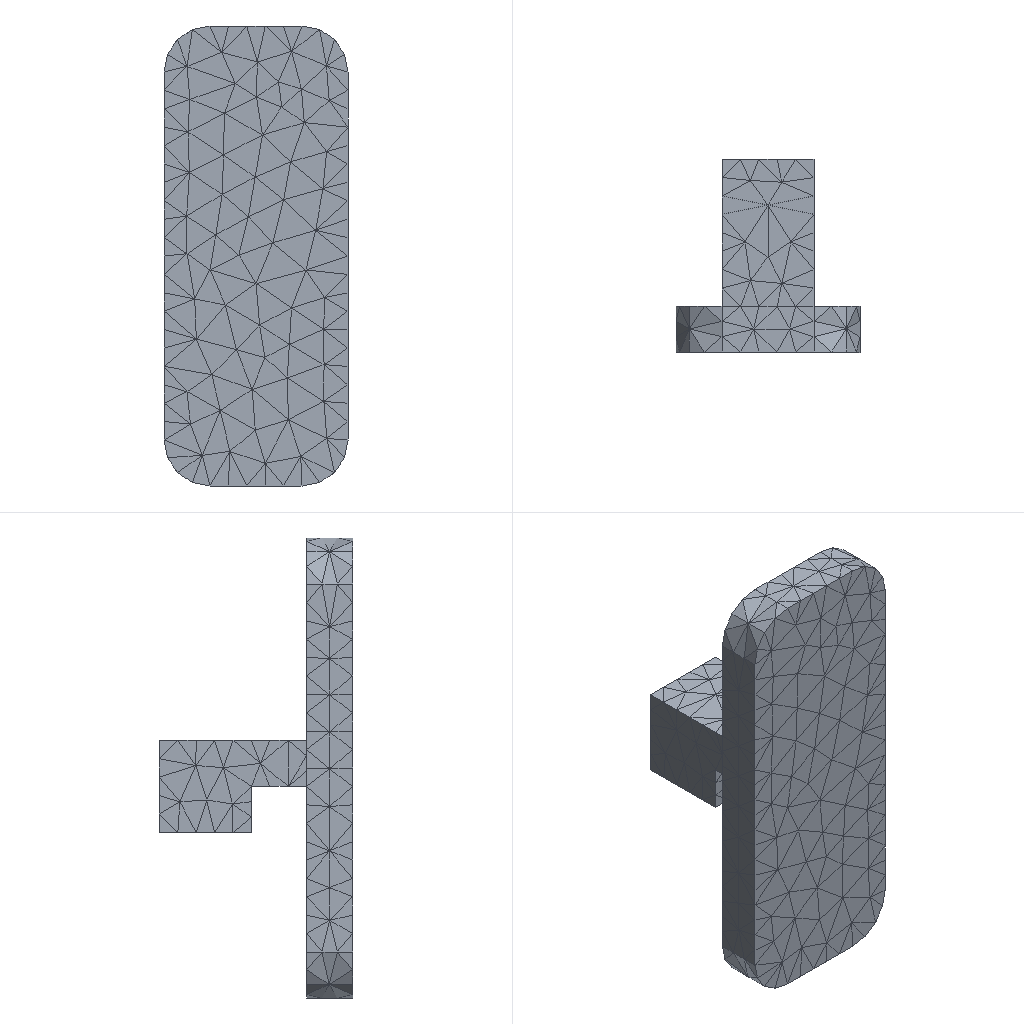Simulation study | ansys workbench
Ansys APDL input file, long lists of numbers shortened:
/batch
/config,noeldb,1     ! force off writing results to database
*get,_wallstrt,active,,time,wall
! ANSYS input file written by Workbench version 2022 R1
! File used for geometry attach:
/title,111111--____ (E5)
! ****** Begin Custom Load Command Snippet ******
/COM, ACT Extensions:
/COM,     LSDYNA, 2021.1
/COM,
! ****** End   Custom Load Command Snippet ******
*DIM,_wb_ProjectScratch_dir,string,248
_wb_ProjectScratch_dir(1) = ''
*DIM,_wb_SolverFiles_dir,string,248
_wb_SolverFiles_dir(1) = ''
*DIM,_wb_userfiles_dir,string,248
_wb_userfiles_dir(1) = ''
/com,--- Data in consistent NMM units. See Solving Units in the help system for more information.
/units,MPA
/nopr
/wb,file,start              !  signify a WB generated input file
/prep7
! Turn off shape checking because checks already performed inside WB mesher.
! See help system for more information.
SHPP,OFF,,NOWARN
/nolist
etcon,set             ! allow ANSYS to choose best KEYOP's for 180x elements, resets any applicable keyopt to MAPDL defaults
/com,*********** Nodes for the whole assembly ***********
nblock,3,,2930
(1i9,3e20.9e3)
        1     5.000000000E+00     2.100000000E+01    -2.200000000E+01
! (2663 more lines like these left out)
-1
/wb,elem,start            !  set before creation of elements
/com,*********** Elements for Body 1 "SYS-4\__" ***********
et,1,187
eblock,19,solid,,1322
(19i9)
        1        1        1        1        0        0        0        0       10        0        1      258      471      370      442     1836     2406     1832     1834
! (2643 more lines like these left out)
-1
/wb,elem,end               !  done creating elements
/com,*********** Send User Defined Coordinate System(s) ***********
csys,0
toffst,273.15,  ! Temperature offset from absolute zero
/com,*********** Set Reference Temperature ***********
tref,22.
/wb,mat,start              !  starting to send materials
/com,*********** Send Materials ***********
Temperature = 'TEMP' ! Temperature
MP,DENS,1,7.85e-09,	! tonne mm^-3
MP,ALPX,1,1.2e-05,	! C^-1
MP,C,1,434000000,	! mm^2 s^-2 C^-1
MP,KXX,1,60.5,	! tonne mm s^-3 C^-1
MP,RSVX,1,0.00017,	! ohm mm
MP,EX,1,200000,	! tonne s^-2 mm^-1
MP,NUXY,1,0.3,
MP,MURX,1,10000,
/wb,mat,end                !  done sending materials
!************************* Model Summary ********************
!SYS-4\__,	304,	matid,	1
!************************* End Model Summary ********************
! get the diagonal of the bounding box. Needed later for other things
*get,_xmin,node,,mnloc,x
*get,_ymin,node,,mnloc,y
*get,_zmin,node,,mnloc,z
*get,_xmax,node,,mxloc,x
*get,_ymax,node,,mxloc,y
*get,_zmax,node,,mxloc,z
_ASMDIAG=(_xmax-_xmin)*(_xmax-_xmin)+(_ymax-_ymin)*(_ymax-_ymin)+(_zmax-_zmin)*(_zmax-_zmin)
_ASMDIAG=SQRT(_ASMDIAG)
/wb,contact,start          !  starting to send contact
/wb,contact,end            !  done creating contacts
/golist
/wb,load,start             !  starting to send loads
/com,*********** Fixed Supports ***********
CMBLOCK,_FIXEDSU,NODE,      431
(8i10)
       145       148       149       150       151       152       155       158
! (53 more lines like these left out)
cmsel,s,_FIXEDSU
d,all,all
nsel,all
/com,*********** Define Force Using Surface Effect Elements ***********
local,12,0,0.,0.,0.,0.,0.,0.
csys,0
et,2,154
eblock,10,,,28
(15i9)
     2125        2        2        2       12       53      391       54       54      752      754       54      750
! (27 more lines like these left out)
-1
esel,s,type,,2
keyop,2,2,1                ! Apply load in local coordinate system
keyop,2,7,1                ! Use original area so load is constant in large deformation
esel,all
/gst,on,on
fini
*get,_numnode,node,0,count
*get,_numelem,elem,0,count
*get, _MAXELEMNUM, elem, 0, NUM, MAX
*get, _MAXNODENUM, node, 0, NUM, MAX
*get, _MAXELEMTYPE, etyp, 0, NUM, MAX
*get, _MAXREALCONST, real, 0, NUM, MAX
/go
/wb,load,end               !  done creating loads
/com,--- Number of total nodes = %_numnode%
/com,--- Number of contact elements = 28
/com,--- Number of spring elements = 0
/com,--- Number of bearing elements = 0
/com,--- Number of solid elements = 1322
/com,--- Number of condensed parts = 0
/com,--- Number of total elements = %_numelem%
*get,_wallbsol,active,,time,wall
/com,****************************************************************************
/com,*************************    SOLUTION       ********************************
/com,****************************************************************************
/solu
antype,0                   ! static analysis
_thickRatio=  0     ! Ratio of thick parts in the model
eqsl,sparse,,,,,1
cntr,print,1               ! print out contact info and also make no initial contact an error
dmpoption,emat,no             ! Don't combine emat file for DANSYS
dmpoption,esav,no             ! Don't combine esav file for DANSYS
nldiag,cont,iter           ! print out contact info each equilibrium iteration
rescontrol,,none                 ! Do not keep any restart files
/com,****************************************************
/com,******************* SOLVE FOR LS 1 OF 1 ****************
esel,s,type,,2
nsle
sfe,all,1,pres,1,0.
sfe,all,2,pres,1,0.
sfe,all,3,pres,1,5.
nsel,all
esel,all
/nopr
/gopr
nsub,1,1,1
time,1.
outres,erase
outres,all,none
outres,nsol,all,
outres,rsol,all
outres,eangl,all
outres,etmp,all
outres,veng,all
outres,strs,all,
outres,epel,all,
outres,eppl,all,
outres,cont,all,
! *********** WB SOLVE COMMAND ***********
! check interactive state
*get,ANSINTER_,active,,int
*if,ANSINTER_,ne,0,then
/eof
*endif
solve
/com *************** Write FE CONNECTORS *********
CEWRITE,file,ce,,INTE
/com,****************************************************
/com,*************** FINISHED SOLVE FOR LS 1 *************
*get,_wallasol,active,,time,wall
/nopr
*get,_numnode,node,0,count
*get,_numelem,elem,0,count
*get, _MAXELEMNUM, elem, 0, NUM, MAX
*get, _MAXNODENUM, node, 0, NUM, MAX,,,INTERNAL
*get, _MAXELEMTYPE, etyp, 0, NUM, MAX
*get, _MAXREALCONST, real, 0, NUM, MAX
/gopr
/post1
xmlo,ENCODING,ISO-8859-1
xmlo,parm
/xml,parm,xml
fini
/gopr
*get,_walldone,active,,time,wall
_preptime=(_wallbsol-_wallstrt)*3600
_solvtime=(_wallasol-_wallbsol)*3600
_posttime=(_walldone-_wallasol)*3600
_totaltim=(_walldone-_wallstrt)*3600
*get,_dlbratio,active,0,solu,dlbr
*get,_combtime,active,0,solu,comb
*get,_ssmode,active,0,solu,ssmm
*get,_ndofs,active,0,solu,ndof
*get,_sol_end_time,active,0,set,time
*if,_sol_end_time,eq,1.,then
/fclean				!clean distributed files
*endif
/com,--- Total number of nodes = %_numnode%
/com,--- Total number of elements = %_numelem%
/com,--- Element load balance ratio = %_dlbratio%
/com,--- Time to combine distributed files = %_combtime%
/com,--- Sparse memory mode = %_ssmode%
/com,--- Number of DOF = %_ndofs%
/wb,file,end               ! done with WB generated input